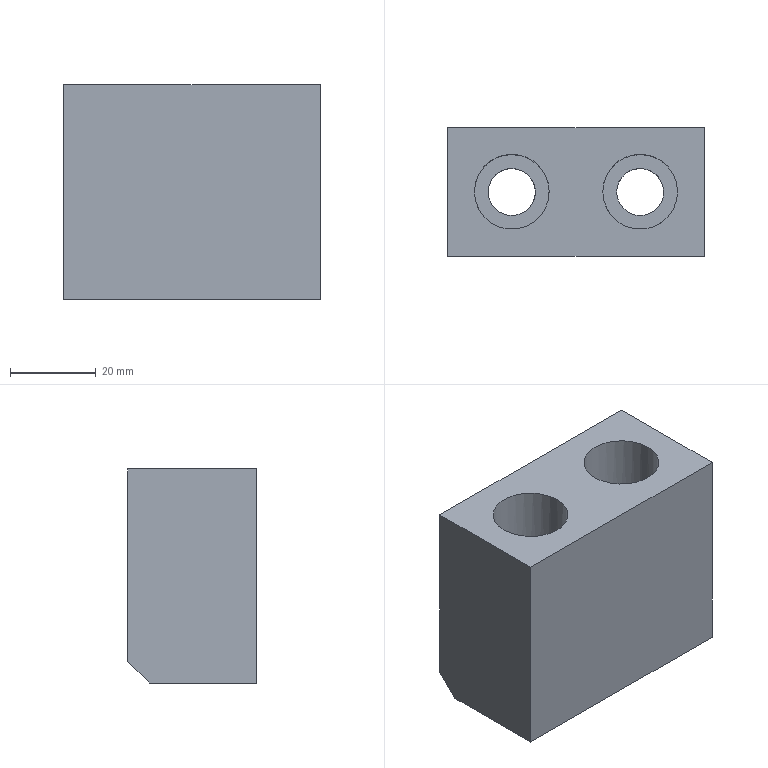Part | NX | features solid 2 | 1 solid | 13 faces | box 60 x 30 x 50 mm | volume 71017 mm3 | plane 9 | cylinder 4 | commonest cylinder face diameters 11 x2 17.5 x2
STEP:
#1=CARTESIAN_POINT('',(341.25,630.,175.));
#2=VERTEX_POINT('',#1);
#3=CARTESIAN_POINT('',(350.,630.,175.));
#4=DIRECTION('',(0.,0.,-1.));
#5=DIRECTION('',(-1.,0.,0.));
#6=AXIS2_PLACEMENT_3D('',#3,#4,#5);
#7=CIRCLE('',#6,8.75);
#8=EDGE_CURVE('',#2,#2,#7,.T.);
#9=ORIENTED_EDGE('',*,*,#8,.T.);
#10=EDGE_LOOP('',(#9));
#11=FACE_BOUND('',#10,.T.);
#12=CARTESIAN_POINT('',(311.25,630.,175.));
#13=VERTEX_POINT('',#12);
#14=CARTESIAN_POINT('',(320.,630.,175.));
#15=DIRECTION('',(0.,0.,-1.));
#16=DIRECTION('',(-1.,0.,0.));
#17=AXIS2_PLACEMENT_3D('',#14,#15,#16);
#18=CIRCLE('',#17,8.75);
#19=EDGE_CURVE('',#13,#13,#18,.T.);
#20=ORIENTED_EDGE('',*,*,#19,.T.);
#21=EDGE_LOOP('',(#20));
#22=FACE_BOUND('',#21,.T.);
#23=CARTESIAN_POINT('',(365.,615.,175.));
#24=VERTEX_POINT('',#23);
#25=CARTESIAN_POINT('',(305.,615.,175.));
#26=VERTEX_POINT('',#25);
#27=CARTESIAN_POINT('',(335.,615.,175.));
#28=DIRECTION('',(-1.,0.,0.));
#29=VECTOR('',#28,1000.);
#30=LINE('',#27,#29);
#31=EDGE_CURVE('',#24,#26,#30,.T.);
#32=ORIENTED_EDGE('',*,*,#31,.F.);
#33=CARTESIAN_POINT('',(365.,645.,175.));
#34=VERTEX_POINT('',#33);
#35=CARTESIAN_POINT('',(365.,630.,175.));
#36=DIRECTION('',(0.,-1.,0.));
#37=VECTOR('',#36,1000.);
#38=LINE('',#35,#37);
#39=EDGE_CURVE('',#34,#24,#38,.T.);
#40=ORIENTED_EDGE('',*,*,#39,.F.);
#41=CARTESIAN_POINT('',(305.,645.,175.));
#42=VERTEX_POINT('',#41);
#43=CARTESIAN_POINT('',(335.,645.,175.));
#44=DIRECTION('',(1.,0.,0.));
#45=VECTOR('',#44,1000.);
#46=LINE('',#43,#45);
#47=EDGE_CURVE('',#42,#34,#46,.T.);
#48=ORIENTED_EDGE('',*,*,#47,.F.);
#49=CARTESIAN_POINT('',(305.,630.,175.));
#50=DIRECTION('',(0.,1.,0.));
#51=VECTOR('',#50,1000.);
#52=LINE('',#49,#51);
#53=EDGE_CURVE('',#26,#42,#52,.T.);
#54=ORIENTED_EDGE('',*,*,#53,.F.);
#55=EDGE_LOOP('',(#32,#40,#48,#54));
#56=FACE_BOUND('',#55,.T.);
#57=CARTESIAN_POINT('',(335.,630.,175.));
#58=DIRECTION('',(0.,0.,1.));
#59=DIRECTION('',(1.,0.,0.));
#60=AXIS2_PLACEMENT_3D('',#57,#58,#59);
#61=PLANE('',#60);
#62=ADVANCED_FACE('',(#11,#22,#56),#61,.T.);
#63=CARTESIAN_POINT('',(365.,615.,125.));
#64=VERTEX_POINT('',#63);
#65=CARTESIAN_POINT('',(365.,615.,125.));
#66=DIRECTION('',(0.,0.,1.));
#67=VECTOR('',#66,1000.);
#68=LINE('',#65,#67);
#69=EDGE_CURVE('',#64,#24,#68,.T.);
#70=ORIENTED_EDGE('',*,*,#69,.T.);
#71=ORIENTED_EDGE('',*,*,#31,.T.);
#72=CARTESIAN_POINT('',(305.,615.,125.));
#73=VERTEX_POINT('',#72);
#74=CARTESIAN_POINT('',(305.,615.,125.));
#75=DIRECTION('',(0.,0.,1.));
#76=VECTOR('',#75,1000.);
#77=LINE('',#74,#76);
#78=EDGE_CURVE('',#73,#26,#77,.T.);
#79=ORIENTED_EDGE('',*,*,#78,.F.);
#80=CARTESIAN_POINT('',(335.,615.,125.));
#81=DIRECTION('',(1.,0.,0.));
#82=VECTOR('',#81,1000.);
#83=LINE('',#80,#82);
#84=EDGE_CURVE('',#73,#64,#83,.T.);
#85=ORIENTED_EDGE('',*,*,#84,.T.);
#86=EDGE_LOOP('',(#70,#71,#79,#85));
#87=FACE_BOUND('',#86,.T.);
#88=CARTESIAN_POINT('',(335.,615.,125.));
#89=DIRECTION('',(0.,-1.,0.));
#90=DIRECTION('',(0.,0.,-1.));
#91=AXIS2_PLACEMENT_3D('',#88,#89,#90);
#92=PLANE('',#91);
#93=ADVANCED_FACE('',(#87),#92,.T.);
#94=CARTESIAN_POINT('',(305.,645.,130.));
#95=VERTEX_POINT('',#94);
#96=CARTESIAN_POINT('',(305.,645.,125.));
#97=DIRECTION('',(0.,0.,1.));
#98=VECTOR('',#97,1000.);
#99=LINE('',#96,#98);
#100=EDGE_CURVE('',#95,#42,#99,.T.);
#101=ORIENTED_EDGE('',*,*,#100,.F.);
#102=CARTESIAN_POINT('',(305.,640.,125.));
#103=VERTEX_POINT('',#102);
#104=CARTESIAN_POINT('',(305.,635.,120.));
#105=DIRECTION('',(0.,0.7071,0.7071));
#106=VECTOR('',#105,1000.);
#107=LINE('',#104,#106);
#108=EDGE_CURVE('',#95,#103,#107,.F.);
#109=ORIENTED_EDGE('',*,*,#108,.T.);
#110=CARTESIAN_POINT('',(305.,630.,125.));
#111=DIRECTION('',(0.,-1.,0.));
#112=VECTOR('',#111,1000.);
#113=LINE('',#110,#112);
#114=EDGE_CURVE('',#103,#73,#113,.T.);
#115=ORIENTED_EDGE('',*,*,#114,.T.);
#116=ORIENTED_EDGE('',*,*,#78,.T.);
#117=ORIENTED_EDGE('',*,*,#53,.T.);
#118=EDGE_LOOP('',(#101,#109,#115,#116,#117));
#119=FACE_BOUND('',#118,.T.);
#120=CARTESIAN_POINT('',(305.,630.,125.));
#121=DIRECTION('',(-1.,0.,0.));
#122=DIRECTION('',(0.,0.,1.));
#123=AXIS2_PLACEMENT_3D('',#120,#121,#122);
#124=PLANE('',#123);
#125=ADVANCED_FACE('',(#119),#124,.T.);
#126=CARTESIAN_POINT('',(365.,645.,130.));
#127=VERTEX_POINT('',#126);
#128=CARTESIAN_POINT('',(365.,645.,125.));
#129=DIRECTION('',(0.,0.,1.));
#130=VECTOR('',#129,1000.);
#131=LINE('',#128,#130);
#132=EDGE_CURVE('',#127,#34,#131,.T.);
#133=ORIENTED_EDGE('',*,*,#132,.F.);
#134=CARTESIAN_POINT('',(335.,645.,130.));
#135=DIRECTION('',(-1.,0.,0.));
#136=VECTOR('',#135,1000.);
#137=LINE('',#134,#136);
#138=EDGE_CURVE('',#127,#95,#137,.T.);
#139=ORIENTED_EDGE('',*,*,#138,.T.);
#140=ORIENTED_EDGE('',*,*,#100,.T.);
#141=ORIENTED_EDGE('',*,*,#47,.T.);
#142=EDGE_LOOP('',(#133,#139,#140,#141));
#143=FACE_BOUND('',#142,.T.);
#144=CARTESIAN_POINT('',(335.,645.,125.));
#145=DIRECTION('',(0.,1.,0.));
#146=DIRECTION('',(0.,0.,1.));
#147=AXIS2_PLACEMENT_3D('',#144,#145,#146);
#148=PLANE('',#147);
#149=ADVANCED_FACE('',(#143),#148,.T.);
#150=CARTESIAN_POINT('',(344.5,630.,125.));
#151=VERTEX_POINT('',#150);
#152=CARTESIAN_POINT('',(350.,630.,125.));
#153=DIRECTION('',(0.,0.,-1.));
#154=DIRECTION('',(-1.,0.,0.));
#155=AXIS2_PLACEMENT_3D('',#152,#153,#154);
#156=CIRCLE('',#155,5.5);
#157=EDGE_CURVE('',#151,#151,#156,.T.);
#158=ORIENTED_EDGE('',*,*,#157,.F.);
#159=EDGE_LOOP('',(#158));
#160=FACE_BOUND('',#159,.T.);
#161=CARTESIAN_POINT('',(314.5,630.,125.));
#162=VERTEX_POINT('',#161);
#163=CARTESIAN_POINT('',(320.,630.,125.));
#164=DIRECTION('',(0.,0.,-1.));
#165=DIRECTION('',(-1.,0.,0.));
#166=AXIS2_PLACEMENT_3D('',#163,#164,#165);
#167=CIRCLE('',#166,5.5);
#168=EDGE_CURVE('',#162,#162,#167,.T.);
#169=ORIENTED_EDGE('',*,*,#168,.F.);
#170=EDGE_LOOP('',(#169));
#171=FACE_BOUND('',#170,.T.);
#172=ORIENTED_EDGE('',*,*,#114,.F.);
#173=CARTESIAN_POINT('',(365.,640.,125.));
#174=VERTEX_POINT('',#173);
#175=CARTESIAN_POINT('',(335.,640.,125.));
#176=DIRECTION('',(1.,0.,0.));
#177=VECTOR('',#176,1000.);
#178=LINE('',#175,#177);
#179=EDGE_CURVE('',#103,#174,#178,.T.);
#180=ORIENTED_EDGE('',*,*,#179,.T.);
#181=CARTESIAN_POINT('',(365.,630.,125.));
#182=DIRECTION('',(0.,1.,0.));
#183=VECTOR('',#182,1000.);
#184=LINE('',#181,#183);
#185=EDGE_CURVE('',#64,#174,#184,.T.);
#186=ORIENTED_EDGE('',*,*,#185,.F.);
#187=ORIENTED_EDGE('',*,*,#84,.F.);
#188=EDGE_LOOP('',(#172,#180,#186,#187));
#189=FACE_BOUND('',#188,.T.);
#190=CARTESIAN_POINT('',(335.,630.,125.));
#191=DIRECTION('',(0.,0.,-1.));
#192=DIRECTION('',(-1.,0.,0.));
#193=AXIS2_PLACEMENT_3D('',#190,#191,#192);
#194=PLANE('',#193);
#195=ADVANCED_FACE('',(#160,#171,#189),#194,.T.);
#196=ORIENTED_EDGE('',*,*,#185,.T.);
#197=CARTESIAN_POINT('',(365.,635.,120.));
#198=DIRECTION('',(0.,-0.7071,-0.7071));
#199=VECTOR('',#198,1000.);
#200=LINE('',#197,#199);
#201=EDGE_CURVE('',#174,#127,#200,.F.);
#202=ORIENTED_EDGE('',*,*,#201,.T.);
#203=ORIENTED_EDGE('',*,*,#132,.T.);
#204=ORIENTED_EDGE('',*,*,#39,.T.);
#205=ORIENTED_EDGE('',*,*,#69,.F.);
#206=EDGE_LOOP('',(#196,#202,#203,#204,#205));
#207=FACE_BOUND('',#206,.T.);
#208=CARTESIAN_POINT('',(365.,630.,125.));
#209=DIRECTION('',(1.,0.,0.));
#210=DIRECTION('',(0.,0.,-1.));
#211=AXIS2_PLACEMENT_3D('',#208,#209,#210);
#212=PLANE('',#211);
#213=ADVANCED_FACE('',(#207),#212,.T.);
#214=ORIENTED_EDGE('',*,*,#168,.T.);
#215=EDGE_LOOP('',(#214));
#216=FACE_BOUND('',#215,.T.);
#217=CARTESIAN_POINT('',(320.,635.5,145.));
#218=VERTEX_POINT('',#217);
#219=CARTESIAN_POINT('',(320.,630.,145.));
#220=DIRECTION('',(0.,0.,-1.));
#221=DIRECTION('',(0.,1.,0.));
#222=AXIS2_PLACEMENT_3D('',#219,#220,#221);
#223=CIRCLE('',#222,5.5);
#224=EDGE_CURVE('',#218,#218,#223,.T.);
#225=ORIENTED_EDGE('',*,*,#224,.F.);
#226=EDGE_LOOP('',(#225));
#227=FACE_BOUND('',#226,.T.);
#228=CARTESIAN_POINT('',(320.,630.,105.));
#229=DIRECTION('',(0.,0.,-1.));
#230=DIRECTION('',(-1.,0.,0.));
#231=AXIS2_PLACEMENT_3D('',#228,#229,#230);
#232=CYLINDRICAL_SURFACE('',#231,5.5);
#233=ADVANCED_FACE('',(#216,#227),#232,.F.);
#234=ORIENTED_EDGE('',*,*,#224,.T.);
#235=EDGE_LOOP('',(#234));
#236=FACE_BOUND('',#235,.T.);
#237=CARTESIAN_POINT('',(320.,638.75,145.));
#238=VERTEX_POINT('',#237);
#239=CARTESIAN_POINT('',(320.,630.,145.));
#240=DIRECTION('',(0.,0.,-1.));
#241=DIRECTION('',(0.,1.,0.));
#242=AXIS2_PLACEMENT_3D('',#239,#240,#241);
#243=CIRCLE('',#242,8.75);
#244=EDGE_CURVE('',#238,#238,#243,.T.);
#245=ORIENTED_EDGE('',*,*,#244,.F.);
#246=EDGE_LOOP('',(#245));
#247=FACE_BOUND('',#246,.T.);
#248=CARTESIAN_POINT('',(320.,630.,145.));
#249=DIRECTION('',(0.,0.,-1.));
#250=DIRECTION('',(-1.,0.,0.));
#251=AXIS2_PLACEMENT_3D('',#248,#249,#250);
#252=PLANE('',#251);
#253=ADVANCED_FACE('',(#236,#247),#252,.F.);
#254=ORIENTED_EDGE('',*,*,#244,.T.);
#255=EDGE_LOOP('',(#254));
#256=FACE_BOUND('',#255,.T.);
#257=ORIENTED_EDGE('',*,*,#19,.F.);
#258=EDGE_LOOP('',(#257));
#259=FACE_BOUND('',#258,.T.);
#260=CARTESIAN_POINT('',(320.,630.,175.));
#261=DIRECTION('',(0.,0.,-1.));
#262=DIRECTION('',(-1.,0.,0.));
#263=AXIS2_PLACEMENT_3D('',#260,#261,#262);
#264=CYLINDRICAL_SURFACE('',#263,8.75);
#265=ADVANCED_FACE('',(#256,#259),#264,.F.);
#266=ORIENTED_EDGE('',*,*,#157,.T.);
#267=EDGE_LOOP('',(#266));
#268=FACE_BOUND('',#267,.T.);
#269=CARTESIAN_POINT('',(350.,635.5,145.));
#270=VERTEX_POINT('',#269);
#271=CARTESIAN_POINT('',(350.,630.,145.));
#272=DIRECTION('',(0.,0.,-1.));
#273=DIRECTION('',(0.,1.,0.));
#274=AXIS2_PLACEMENT_3D('',#271,#272,#273);
#275=CIRCLE('',#274,5.5);
#276=EDGE_CURVE('',#270,#270,#275,.T.);
#277=ORIENTED_EDGE('',*,*,#276,.F.);
#278=EDGE_LOOP('',(#277));
#279=FACE_BOUND('',#278,.T.);
#280=CARTESIAN_POINT('',(350.,630.,105.));
#281=DIRECTION('',(0.,0.,-1.));
#282=DIRECTION('',(-1.,0.,0.));
#283=AXIS2_PLACEMENT_3D('',#280,#281,#282);
#284=CYLINDRICAL_SURFACE('',#283,5.5);
#285=ADVANCED_FACE('',(#268,#279),#284,.F.);
#286=ORIENTED_EDGE('',*,*,#276,.T.);
#287=EDGE_LOOP('',(#286));
#288=FACE_BOUND('',#287,.T.);
#289=CARTESIAN_POINT('',(350.,638.75,145.));
#290=VERTEX_POINT('',#289);
#291=CARTESIAN_POINT('',(350.,630.,145.));
#292=DIRECTION('',(0.,0.,-1.));
#293=DIRECTION('',(0.,1.,0.));
#294=AXIS2_PLACEMENT_3D('',#291,#292,#293);
#295=CIRCLE('',#294,8.75);
#296=EDGE_CURVE('',#290,#290,#295,.T.);
#297=ORIENTED_EDGE('',*,*,#296,.F.);
#298=EDGE_LOOP('',(#297));
#299=FACE_BOUND('',#298,.T.);
#300=CARTESIAN_POINT('',(350.,630.,145.));
#301=DIRECTION('',(0.,0.,-1.));
#302=DIRECTION('',(-1.,0.,0.));
#303=AXIS2_PLACEMENT_3D('',#300,#301,#302);
#304=PLANE('',#303);
#305=ADVANCED_FACE('',(#288,#299),#304,.F.);
#306=ORIENTED_EDGE('',*,*,#296,.T.);
#307=EDGE_LOOP('',(#306));
#308=FACE_BOUND('',#307,.T.);
#309=ORIENTED_EDGE('',*,*,#8,.F.);
#310=EDGE_LOOP('',(#309));
#311=FACE_BOUND('',#310,.T.);
#312=CARTESIAN_POINT('',(350.,630.,175.));
#313=DIRECTION('',(0.,0.,-1.));
#314=DIRECTION('',(-1.,0.,0.));
#315=AXIS2_PLACEMENT_3D('',#312,#313,#314);
#316=CYLINDRICAL_SURFACE('',#315,8.75);
#317=ADVANCED_FACE('',(#308,#311),#316,.F.);
#318=ORIENTED_EDGE('',*,*,#201,.F.);
#319=ORIENTED_EDGE('',*,*,#179,.F.);
#320=ORIENTED_EDGE('',*,*,#108,.F.);
#321=ORIENTED_EDGE('',*,*,#138,.F.);
#322=EDGE_LOOP('',(#318,#319,#320,#321));
#323=FACE_BOUND('',#322,.T.);
#324=CARTESIAN_POINT('',(335.,645.,130.));
#325=DIRECTION('',(0.,-0.7071,0.7071));
#326=DIRECTION('',(0.,-0.7071,-0.7071));
#327=AXIS2_PLACEMENT_3D('',#324,#325,#326);
#328=PLANE('',#327);
#329=ADVANCED_FACE('',(#323),#328,.F.);
#330=CLOSED_SHELL('',(#62,#93,#125,#149,#195,#213,#233,#253,#265,#285,#305,#317,#329));
#331=MANIFOLD_SOLID_BREP('',#330);
#332=(LENGTH_UNIT()NAMED_UNIT(*)SI_UNIT(.MILLI.,.METRE.));
#333=UNCERTAINTY_MEASURE_WITH_UNIT(LENGTH_MEASURE(0.00001),#332,'','');
#334=(NAMED_UNIT(*)PLANE_ANGLE_UNIT()SI_UNIT($,.RADIAN.));
#335=(NAMED_UNIT(*)SI_UNIT($,.STERADIAN.)SOLID_ANGLE_UNIT());
#336=(GEOMETRIC_REPRESENTATION_CONTEXT(3)GLOBAL_UNCERTAINTY_ASSIGNED_CONTEXT((#333))GLOBAL_UNIT_ASSIGNED_CONTEXT((#332,#334,#335))REPRESENTATION_CONTEXT('',''));
#337=ADVANCED_BREP_SHAPE_REPRESENTATION('',(#331),#336);